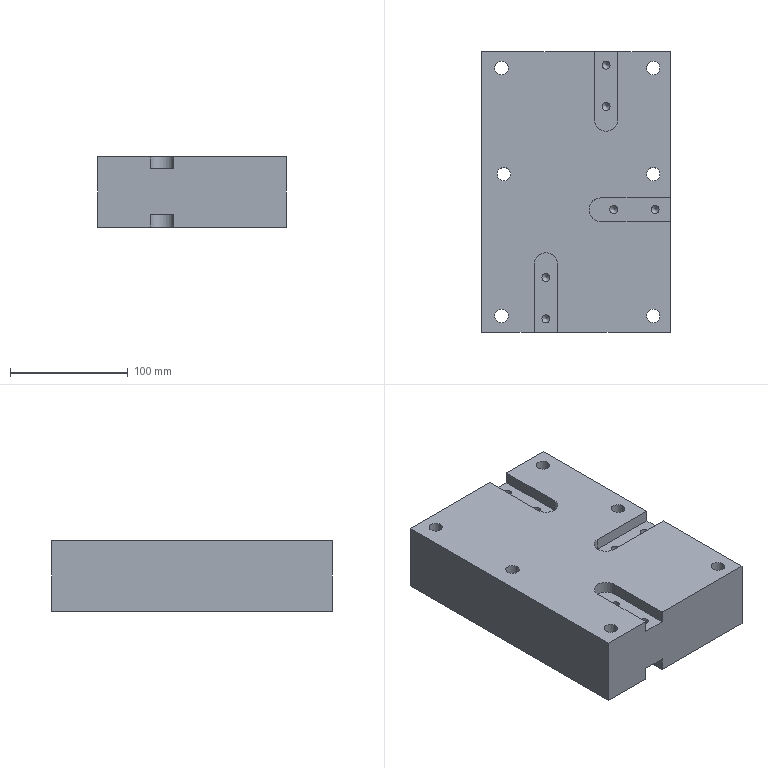Part | NX | features 23 2 | 1 solid | 56 faces | box 160 x 238 x 59.5 mm | volume 2139878 mm3 | cylinder 26 | plane 24 | cone 6 | commonest cylinder face diameters 20 x14 6.8 x6 11.5 x6